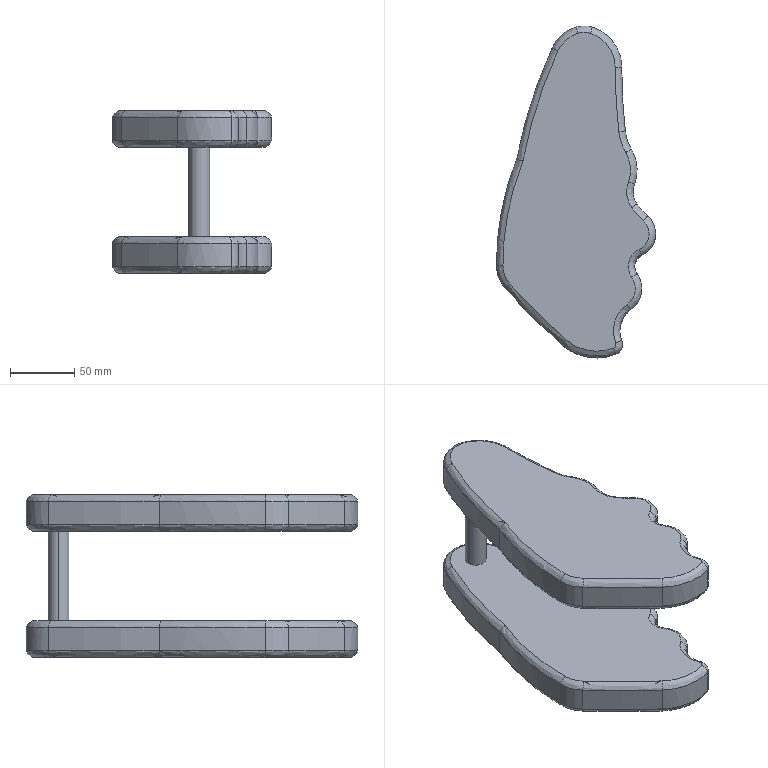Part | SolidWorks | features Extrusion 1, Fillet 1, ICE 1, MirrorSolid 1 | 1 solid | 120 faces | box 124.14 x 258.791 x 126.388 mm | volume 1203274 mm3 | spline 72 | cylinder 44 | plane 4 | commonest cylinder face diameters 19.194 x4 33.861 x4 40.717 x4 16.213 x2 16.256 x2 36.989 x2